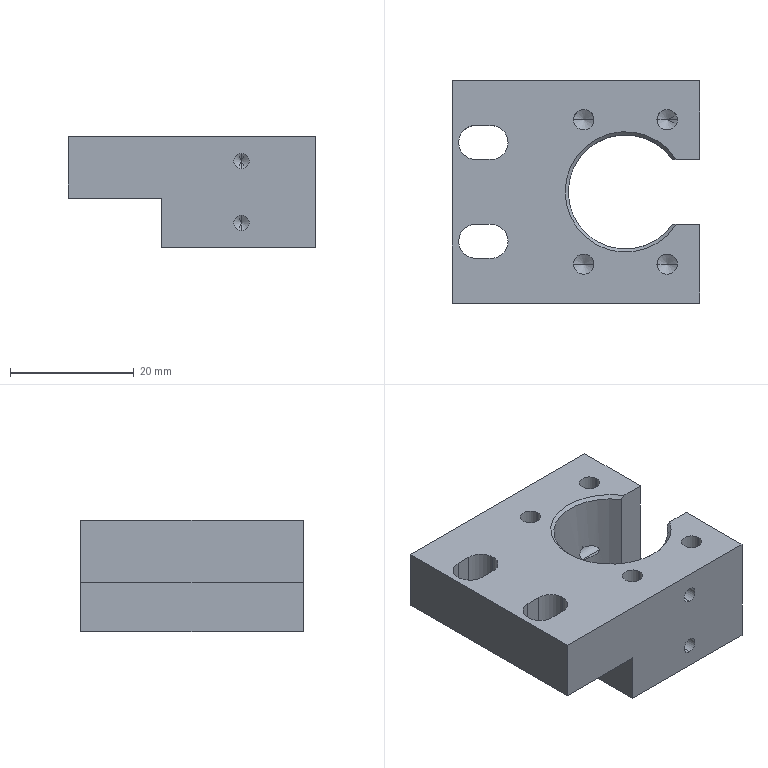Part | NX | features BREP 1 | 1 solid | 68 faces | box 40 x 36 x 18 mm | volume 14715 mm3 | cylinder 28 | cone 25 | plane 15 | commonest cylinder face diameters 2.5 x12 3.3 x8 5.5 x6 18.5 x2